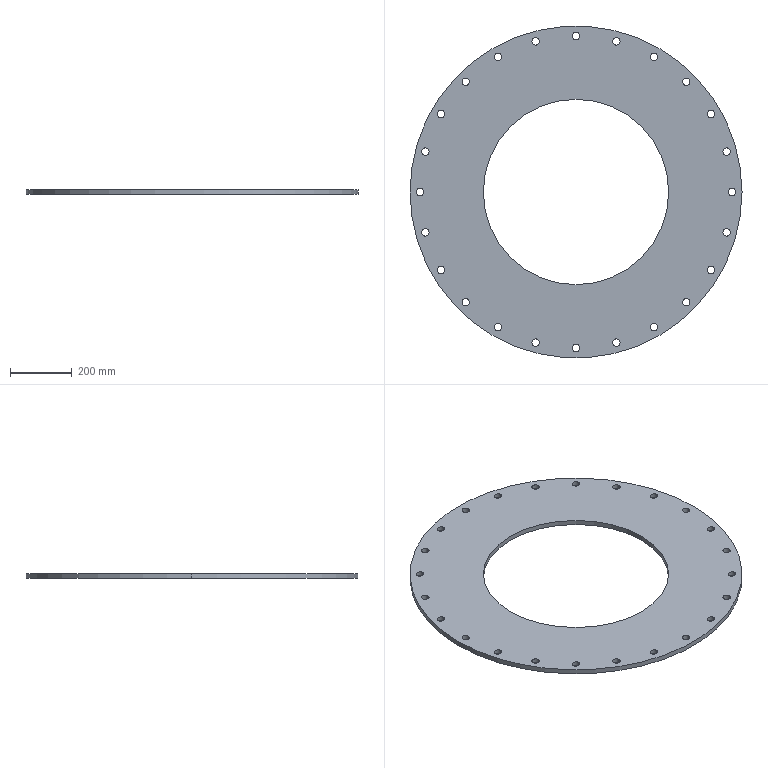Part | SolidWorks | features CirPattern 1, FlatPattern 1, HoleWzd 1, ICE 1, SMBaseFlange 1, SheetMetal 1 | 1 solid | 54 faces | box 1075 x 1075 x 16 mm | volume 9824401 mm3 | cylinder 52 | plane 2 | commonest cylinder face diameters 24 x48 600 x2 1075 x2